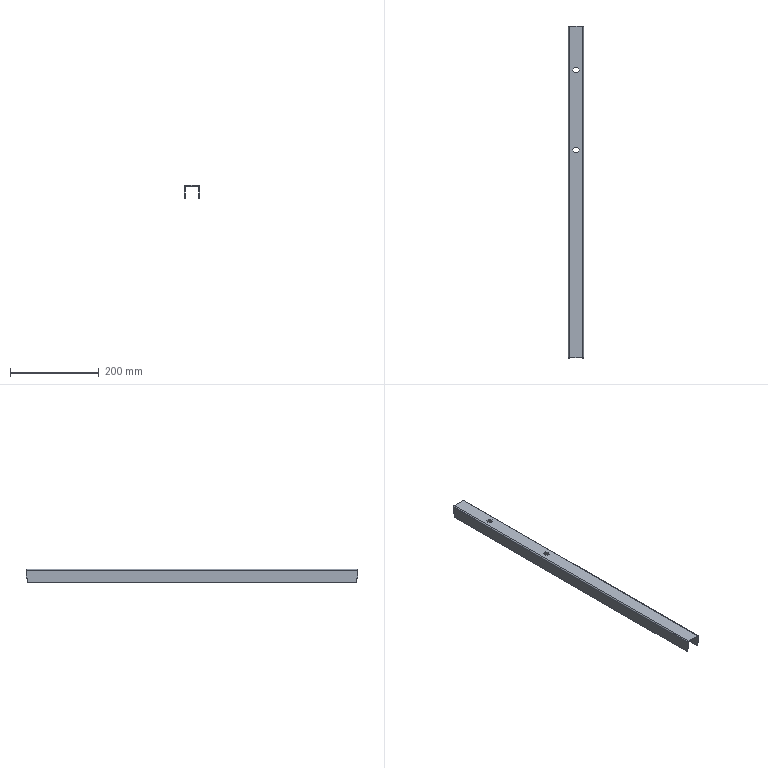Part | SolidWorks | features BaseBody 1 | 1 solid | 42 faces | box 34 x 750 x 29.5 mm | volume 130830 mm3 | plane 38 | cylinder 4 | commonest cylinder face diameters 1 x2 5 x2
STEP:
#1=CARTESIAN_POINT('',(-15.,372.,-29.5));
#2=VERTEX_POINT('',#1);
#3=CARTESIAN_POINT('',(-17.,372.,-29.5));
#4=VERTEX_POINT('',#3);
#5=CARTESIAN_POINT('',(17.,372.,-29.5));
#6=DIRECTION('',(-1.,0.,0.));
#7=VECTOR('',#6,1000.);
#8=LINE('',#5,#7);
#9=EDGE_CURVE('',#2,#4,#8,.T.);
#10=ORIENTED_EDGE('',*,*,#9,.T.);
#11=CARTESIAN_POINT('',(-17.,372.,-19.5));
#12=VERTEX_POINT('',#11);
#13=CARTESIAN_POINT('',(-17.,372.,-29.5));
#14=DIRECTION('',(0.,0.,1.));
#15=VECTOR('',#14,1000.);
#16=LINE('',#13,#15);
#17=EDGE_CURVE('',#4,#12,#16,.T.);
#18=ORIENTED_EDGE('',*,*,#17,.T.);
#19=CARTESIAN_POINT('',(-15.,372.,-19.5));
#20=VERTEX_POINT('',#19);
#21=CARTESIAN_POINT('',(17.,372.,-19.5));
#22=DIRECTION('',(-1.,0.,0.));
#23=VECTOR('',#22,1000.);
#24=LINE('',#21,#23);
#25=EDGE_CURVE('',#20,#12,#24,.T.);
#26=ORIENTED_EDGE('',*,*,#25,.F.);
#27=CARTESIAN_POINT('',(-15.,372.,0.));
#28=DIRECTION('',(0.,0.,1.));
#29=VECTOR('',#28,1000.);
#30=LINE('',#27,#29);
#31=EDGE_CURVE('',#2,#20,#30,.T.);
#32=ORIENTED_EDGE('',*,*,#31,.F.);
#33=EDGE_LOOP('',(#10,#18,#26,#32));
#34=FACE_OUTER_BOUND('',#33,.T.);
#35=CARTESIAN_POINT('',(17.,372.,-29.5));
#36=DIRECTION('',(0.,-1.,0.));
#37=DIRECTION('',(0.,0.,-1.));
#38=AXIS2_PLACEMENT_3D('',#35,#36,#37);
#39=PLANE('',#38);
#40=ADVANCED_FACE('',(#34),#39,.F.);
#41=ORIENTED_EDGE('',*,*,#25,.T.);
#42=CARTESIAN_POINT('',(-17.,375.,-19.5));
#43=VERTEX_POINT('',#42);
#44=CARTESIAN_POINT('',(-17.,375.,-19.5));
#45=DIRECTION('',(0.,1.,0.));
#46=VECTOR('',#45,1000.);
#47=LINE('',#44,#46);
#48=EDGE_CURVE('',#12,#43,#47,.T.);
#49=ORIENTED_EDGE('',*,*,#48,.T.);
#50=CARTESIAN_POINT('',(-15.,375.,-19.5));
#51=VERTEX_POINT('',#50);
#52=CARTESIAN_POINT('',(17.,375.,-19.5));
#53=DIRECTION('',(-1.,0.,0.));
#54=VECTOR('',#53,1000.);
#55=LINE('',#52,#54);
#56=EDGE_CURVE('',#51,#43,#55,.T.);
#57=ORIENTED_EDGE('',*,*,#56,.F.);
#58=CARTESIAN_POINT('',(-15.,0.,-19.5));
#59=DIRECTION('',(0.,1.,0.));
#60=VECTOR('',#59,1000.);
#61=LINE('',#58,#60);
#62=EDGE_CURVE('',#20,#51,#61,.T.);
#63=ORIENTED_EDGE('',*,*,#62,.F.);
#64=EDGE_LOOP('',(#41,#49,#57,#63));
#65=FACE_OUTER_BOUND('',#64,.T.);
#66=CARTESIAN_POINT('',(17.,375.,-19.5));
#67=DIRECTION('',(0.,0.,1.));
#68=DIRECTION('',(1.,0.,0.));
#69=AXIS2_PLACEMENT_3D('',#66,#67,#68);
#70=PLANE('',#69);
#71=ADVANCED_FACE('',(#65),#70,.F.);
#72=CARTESIAN_POINT('',(-15.,-372.,-19.5));
#73=VERTEX_POINT('',#72);
#74=CARTESIAN_POINT('',(-17.,-372.,-19.5));
#75=VERTEX_POINT('',#74);
#76=CARTESIAN_POINT('',(17.,-372.,-19.5));
#77=DIRECTION('',(-1.,0.,0.));
#78=VECTOR('',#77,1000.);
#79=LINE('',#76,#78);
#80=EDGE_CURVE('',#73,#75,#79,.T.);
#81=ORIENTED_EDGE('',*,*,#80,.T.);
#82=CARTESIAN_POINT('',(-17.,-372.,-29.5));
#83=VERTEX_POINT('',#82);
#84=CARTESIAN_POINT('',(-17.,-372.,-29.5));
#85=DIRECTION('',(0.,0.,-1.));
#86=VECTOR('',#85,1000.);
#87=LINE('',#84,#86);
#88=EDGE_CURVE('',#75,#83,#87,.T.);
#89=ORIENTED_EDGE('',*,*,#88,.T.);
#90=CARTESIAN_POINT('',(-15.,-372.,-29.5));
#91=VERTEX_POINT('',#90);
#92=CARTESIAN_POINT('',(17.,-372.,-29.5));
#93=DIRECTION('',(-1.,0.,0.));
#94=VECTOR('',#93,1000.);
#95=LINE('',#92,#94);
#96=EDGE_CURVE('',#91,#83,#95,.T.);
#97=ORIENTED_EDGE('',*,*,#96,.F.);
#98=CARTESIAN_POINT('',(-15.,-372.,0.));
#99=DIRECTION('',(0.,0.,-1.));
#100=VECTOR('',#99,1000.);
#101=LINE('',#98,#100);
#102=EDGE_CURVE('',#73,#91,#101,.T.);
#103=ORIENTED_EDGE('',*,*,#102,.F.);
#104=EDGE_LOOP('',(#81,#89,#97,#103));
#105=FACE_OUTER_BOUND('',#104,.T.);
#106=CARTESIAN_POINT('',(17.,-372.,-29.5));
#107=DIRECTION('',(0.,1.,0.));
#108=DIRECTION('',(1.,0.,0.));
#109=AXIS2_PLACEMENT_3D('',#106,#107,#108);
#110=PLANE('',#109);
#111=ADVANCED_FACE('',(#105),#110,.F.);
#112=CARTESIAN_POINT('',(-15.,-375.,-19.5));
#113=VERTEX_POINT('',#112);
#114=CARTESIAN_POINT('',(-17.,-375.,-19.5));
#115=VERTEX_POINT('',#114);
#116=CARTESIAN_POINT('',(17.,-375.,-19.5));
#117=DIRECTION('',(-1.,0.,0.));
#118=VECTOR('',#117,1000.);
#119=LINE('',#116,#118);
#120=EDGE_CURVE('',#113,#115,#119,.T.);
#121=ORIENTED_EDGE('',*,*,#120,.T.);
#122=CARTESIAN_POINT('',(-17.,-375.,-19.5));
#123=DIRECTION('',(0.,1.,0.));
#124=VECTOR('',#123,1000.);
#125=LINE('',#122,#124);
#126=EDGE_CURVE('',#115,#75,#125,.T.);
#127=ORIENTED_EDGE('',*,*,#126,.T.);
#128=ORIENTED_EDGE('',*,*,#80,.F.);
#129=CARTESIAN_POINT('',(-15.,0.,-19.5));
#130=DIRECTION('',(0.,1.,0.));
#131=VECTOR('',#130,1000.);
#132=LINE('',#129,#131);
#133=EDGE_CURVE('',#113,#73,#132,.T.);
#134=ORIENTED_EDGE('',*,*,#133,.F.);
#135=EDGE_LOOP('',(#121,#127,#128,#134));
#136=FACE_OUTER_BOUND('',#135,.T.);
#137=CARTESIAN_POINT('',(17.,-375.,-19.5));
#138=DIRECTION('',(0.,0.,1.));
#139=DIRECTION('',(1.,0.,0.));
#140=AXIS2_PLACEMENT_3D('',#137,#138,#139);
#141=PLANE('',#140);
#142=ADVANCED_FACE('',(#136),#141,.F.);
#143=CARTESIAN_POINT('',(15.,372.,-19.5));
#144=VERTEX_POINT('',#143);
#145=CARTESIAN_POINT('',(15.,375.,-19.5));
#146=VERTEX_POINT('',#145);
#147=CARTESIAN_POINT('',(15.,0.,-19.5));
#148=DIRECTION('',(0.,1.,0.));
#149=VECTOR('',#148,1000.);
#150=LINE('',#147,#149);
#151=EDGE_CURVE('',#144,#146,#150,.T.);
#152=ORIENTED_EDGE('',*,*,#151,.T.);
#153=CARTESIAN_POINT('',(17.,375.,-19.5));
#154=VERTEX_POINT('',#153);
#155=CARTESIAN_POINT('',(17.,375.,-19.5));
#156=DIRECTION('',(-1.,0.,0.));
#157=VECTOR('',#156,1000.);
#158=LINE('',#155,#157);
#159=EDGE_CURVE('',#154,#146,#158,.T.);
#160=ORIENTED_EDGE('',*,*,#159,.F.);
#161=CARTESIAN_POINT('',(17.,372.,-19.5));
#162=VERTEX_POINT('',#161);
#163=CARTESIAN_POINT('',(17.,375.,-19.5));
#164=DIRECTION('',(0.,1.,0.));
#165=VECTOR('',#164,1000.);
#166=LINE('',#163,#165);
#167=EDGE_CURVE('',#162,#154,#166,.T.);
#168=ORIENTED_EDGE('',*,*,#167,.F.);
#169=CARTESIAN_POINT('',(17.,372.,-19.5));
#170=DIRECTION('',(-1.,0.,0.));
#171=VECTOR('',#170,1000.);
#172=LINE('',#169,#171);
#173=EDGE_CURVE('',#162,#144,#172,.T.);
#174=ORIENTED_EDGE('',*,*,#173,.T.);
#175=EDGE_LOOP('',(#152,#160,#168,#174));
#176=FACE_OUTER_BOUND('',#175,.T.);
#177=CARTESIAN_POINT('',(17.,375.,-19.5));
#178=DIRECTION('',(0.,0.,1.));
#179=DIRECTION('',(1.,0.,0.));
#180=AXIS2_PLACEMENT_3D('',#177,#178,#179);
#181=PLANE('',#180);
#182=ADVANCED_FACE('',(#176),#181,.F.);
#183=CARTESIAN_POINT('',(15.,372.,-29.5));
#184=VERTEX_POINT('',#183);
#185=CARTESIAN_POINT('',(15.,372.,0.));
#186=DIRECTION('',(0.,0.,1.));
#187=VECTOR('',#186,1000.);
#188=LINE('',#185,#187);
#189=EDGE_CURVE('',#184,#144,#188,.T.);
#190=ORIENTED_EDGE('',*,*,#189,.T.);
#191=ORIENTED_EDGE('',*,*,#173,.F.);
#192=CARTESIAN_POINT('',(17.,372.,-29.5));
#193=VERTEX_POINT('',#192);
#194=CARTESIAN_POINT('',(17.,372.,-29.5));
#195=DIRECTION('',(0.,0.,1.));
#196=VECTOR('',#195,1000.);
#197=LINE('',#194,#196);
#198=EDGE_CURVE('',#193,#162,#197,.T.);
#199=ORIENTED_EDGE('',*,*,#198,.F.);
#200=CARTESIAN_POINT('',(17.,372.,-29.5));
#201=DIRECTION('',(-1.,0.,0.));
#202=VECTOR('',#201,1000.);
#203=LINE('',#200,#202);
#204=EDGE_CURVE('',#193,#184,#203,.T.);
#205=ORIENTED_EDGE('',*,*,#204,.T.);
#206=EDGE_LOOP('',(#190,#191,#199,#205));
#207=FACE_OUTER_BOUND('',#206,.T.);
#208=CARTESIAN_POINT('',(17.,372.,-29.5));
#209=DIRECTION('',(0.,-1.,0.));
#210=DIRECTION('',(0.,0.,-1.));
#211=AXIS2_PLACEMENT_3D('',#208,#209,#210);
#212=PLANE('',#211);
#213=ADVANCED_FACE('',(#207),#212,.F.);
#214=CARTESIAN_POINT('',(15.,-375.,-19.5));
#215=VERTEX_POINT('',#214);
#216=CARTESIAN_POINT('',(15.,-372.,-19.5));
#217=VERTEX_POINT('',#216);
#218=CARTESIAN_POINT('',(15.,0.,-19.5));
#219=DIRECTION('',(0.,1.,0.));
#220=VECTOR('',#219,1000.);
#221=LINE('',#218,#220);
#222=EDGE_CURVE('',#215,#217,#221,.T.);
#223=ORIENTED_EDGE('',*,*,#222,.T.);
#224=CARTESIAN_POINT('',(17.,-372.,-19.5));
#225=VERTEX_POINT('',#224);
#226=CARTESIAN_POINT('',(17.,-372.,-19.5));
#227=DIRECTION('',(-1.,0.,0.));
#228=VECTOR('',#227,1000.);
#229=LINE('',#226,#228);
#230=EDGE_CURVE('',#225,#217,#229,.T.);
#231=ORIENTED_EDGE('',*,*,#230,.F.);
#232=CARTESIAN_POINT('',(17.,-375.,-19.5));
#233=VERTEX_POINT('',#232);
#234=CARTESIAN_POINT('',(17.,-375.,-19.5));
#235=DIRECTION('',(0.,1.,0.));
#236=VECTOR('',#235,1000.);
#237=LINE('',#234,#236);
#238=EDGE_CURVE('',#233,#225,#237,.T.);
#239=ORIENTED_EDGE('',*,*,#238,.F.);
#240=CARTESIAN_POINT('',(17.,-375.,-19.5));
#241=DIRECTION('',(-1.,0.,0.));
#242=VECTOR('',#241,1000.);
#243=LINE('',#240,#242);
#244=EDGE_CURVE('',#233,#215,#243,.T.);
#245=ORIENTED_EDGE('',*,*,#244,.T.);
#246=EDGE_LOOP('',(#223,#231,#239,#245));
#247=FACE_OUTER_BOUND('',#246,.T.);
#248=CARTESIAN_POINT('',(17.,-375.,-19.5));
#249=DIRECTION('',(0.,0.,1.));
#250=DIRECTION('',(1.,0.,0.));
#251=AXIS2_PLACEMENT_3D('',#248,#249,#250);
#252=PLANE('',#251);
#253=ADVANCED_FACE('',(#247),#252,.F.);
#254=CARTESIAN_POINT('',(15.,-372.,-29.5));
#255=VERTEX_POINT('',#254);
#256=CARTESIAN_POINT('',(15.,-372.,0.));
#257=DIRECTION('',(0.,0.,-1.));
#258=VECTOR('',#257,1000.);
#259=LINE('',#256,#258);
#260=EDGE_CURVE('',#217,#255,#259,.T.);
#261=ORIENTED_EDGE('',*,*,#260,.T.);
#262=CARTESIAN_POINT('',(17.,-372.,-29.5));
#263=VERTEX_POINT('',#262);
#264=CARTESIAN_POINT('',(17.,-372.,-29.5));
#265=DIRECTION('',(-1.,0.,0.));
#266=VECTOR('',#265,1000.);
#267=LINE('',#264,#266);
#268=EDGE_CURVE('',#263,#255,#267,.T.);
#269=ORIENTED_EDGE('',*,*,#268,.F.);
#270=CARTESIAN_POINT('',(17.,-372.,-29.5));
#271=DIRECTION('',(0.,0.,-1.));
#272=VECTOR('',#271,1000.);
#273=LINE('',#270,#272);
#274=EDGE_CURVE('',#225,#263,#273,.T.);
#275=ORIENTED_EDGE('',*,*,#274,.F.);
#276=ORIENTED_EDGE('',*,*,#230,.T.);
#277=EDGE_LOOP('',(#261,#269,#275,#276));
#278=FACE_OUTER_BOUND('',#277,.T.);
#279=CARTESIAN_POINT('',(17.,-372.,-29.5));
#280=DIRECTION('',(0.,1.,0.));
#281=DIRECTION('',(1.,0.,0.));
#282=AXIS2_PLACEMENT_3D('',#279,#280,#281);
#283=PLANE('',#282);
#284=ADVANCED_FACE('',(#278),#283,.F.);
#285=CARTESIAN_POINT('',(6.928,275.,0.));
#286=VERTEX_POINT('',#285);
#287=CARTESIAN_POINT('',(3.464,281.,0.));
#288=VERTEX_POINT('',#287);
#289=CARTESIAN_POINT('',(6.928,275.,0.));
#290=DIRECTION('',(-0.5,0.866,0.));
#291=VECTOR('',#290,1000.);
#292=LINE('',#289,#291);
#293=EDGE_CURVE('',#286,#288,#292,.T.);
#294=ORIENTED_EDGE('',*,*,#293,.T.);
#295=CARTESIAN_POINT('',(3.464,281.,-2.));
#296=VERTEX_POINT('',#295);
#297=CARTESIAN_POINT('',(3.464,281.,-2.));
#298=DIRECTION('',(0.,0.,1.));
#299=VECTOR('',#298,1000.);
#300=LINE('',#297,#299);
#301=EDGE_CURVE('',#296,#288,#300,.T.);
#302=ORIENTED_EDGE('',*,*,#301,.F.);
#303=CARTESIAN_POINT('',(6.928,275.,-2.));
#304=VERTEX_POINT('',#303);
#305=CARTESIAN_POINT('',(6.928,275.,-2.));
#306=DIRECTION('',(-0.5,0.866,0.));
#307=VECTOR('',#306,1000.);
#308=LINE('',#305,#307);
#309=EDGE_CURVE('',#304,#296,#308,.T.);
#310=ORIENTED_EDGE('',*,*,#309,.F.);
#311=CARTESIAN_POINT('',(6.928,275.,-2.));
#312=DIRECTION('',(0.,0.,1.));
#313=VECTOR('',#312,1000.);
#314=LINE('',#311,#313);
#315=EDGE_CURVE('',#304,#286,#314,.T.);
#316=ORIENTED_EDGE('',*,*,#315,.T.);
#317=EDGE_LOOP('',(#294,#302,#310,#316));
#318=FACE_OUTER_BOUND('',#317,.T.);
#319=CARTESIAN_POINT('',(6.928,275.,-2.));
#320=DIRECTION('',(0.866,0.5,0.));
#321=DIRECTION('',(0.,0.,-1.));
#322=AXIS2_PLACEMENT_3D('',#319,#320,#321);
#323=PLANE('',#322);
#324=ADVANCED_FACE('',(#318),#323,.F.);
#325=CARTESIAN_POINT('',(-3.464,281.,0.));
#326=VERTEX_POINT('',#325);
#327=CARTESIAN_POINT('',(3.464,281.,0.));
#328=DIRECTION('',(-1.,0.,0.));
#329=VECTOR('',#328,1000.);
#330=LINE('',#327,#329);
#331=EDGE_CURVE('',#288,#326,#330,.T.);
#332=ORIENTED_EDGE('',*,*,#331,.T.);
#333=CARTESIAN_POINT('',(-3.464,281.,-2.));
#334=VERTEX_POINT('',#333);
#335=CARTESIAN_POINT('',(-3.464,281.,-2.));
#336=DIRECTION('',(0.,0.,1.));
#337=VECTOR('',#336,1000.);
#338=LINE('',#335,#337);
#339=EDGE_CURVE('',#334,#326,#338,.T.);
#340=ORIENTED_EDGE('',*,*,#339,.F.);
#341=CARTESIAN_POINT('',(3.464,281.,-2.));
#342=DIRECTION('',(-1.,0.,0.));
#343=VECTOR('',#342,1000.);
#344=LINE('',#341,#343);
#345=EDGE_CURVE('',#296,#334,#344,.T.);
#346=ORIENTED_EDGE('',*,*,#345,.F.);
#347=ORIENTED_EDGE('',*,*,#301,.T.);
#348=EDGE_LOOP('',(#332,#340,#346,#347));
#349=FACE_OUTER_BOUND('',#348,.T.);
#350=CARTESIAN_POINT('',(3.464,281.,-2.));
#351=DIRECTION('',(0.,1.,0.));
#352=DIRECTION('',(1.,0.,0.));
#353=AXIS2_PLACEMENT_3D('',#350,#351,#352);
#354=PLANE('',#353);
#355=ADVANCED_FACE('',(#349),#354,.F.);
#356=CARTESIAN_POINT('',(-6.928,275.,0.));
#357=VERTEX_POINT('',#356);
#358=CARTESIAN_POINT('',(-3.464,281.,0.));
#359=DIRECTION('',(-0.5,-0.866,0.));
#360=VECTOR('',#359,1000.);
#361=LINE('',#358,#360);
#362=EDGE_CURVE('',#326,#357,#361,.T.);
#363=ORIENTED_EDGE('',*,*,#362,.T.);
#364=CARTESIAN_POINT('',(-6.928,275.,-2.));
#365=VERTEX_POINT('',#364);
#366=CARTESIAN_POINT('',(-6.928,275.,-2.));
#367=DIRECTION('',(0.,0.,1.));
#368=VECTOR('',#367,1000.);
#369=LINE('',#366,#368);
#370=EDGE_CURVE('',#365,#357,#369,.T.);
#371=ORIENTED_EDGE('',*,*,#370,.F.);
#372=CARTESIAN_POINT('',(-3.464,281.,-2.));
#373=DIRECTION('',(-0.5,-0.866,0.));
#374=VECTOR('',#373,1000.);
#375=LINE('',#372,#374);
#376=EDGE_CURVE('',#334,#365,#375,.T.);
#377=ORIENTED_EDGE('',*,*,#376,.F.);
#378=ORIENTED_EDGE('',*,*,#339,.T.);
#379=EDGE_LOOP('',(#363,#371,#377,#378));
#380=FACE_OUTER_BOUND('',#379,.T.);
#381=CARTESIAN_POINT('',(-3.464,281.,-2.));
#382=DIRECTION('',(-0.866,0.5,0.));
#383=DIRECTION('',(0.,0.,1.));
#384=AXIS2_PLACEMENT_3D('',#381,#382,#383);
#385=PLANE('',#384);
#386=ADVANCED_FACE('',(#380),#385,.F.);
#387=CARTESIAN_POINT('',(-3.464,269.,0.));
#388=VERTEX_POINT('',#387);
#389=CARTESIAN_POINT('',(-6.928,275.,0.));
#390=DIRECTION('',(0.5,-0.866,0.));
#391=VECTOR('',#390,1000.);
#392=LINE('',#389,#391);
#393=EDGE_CURVE('',#357,#388,#392,.T.);
#394=ORIENTED_EDGE('',*,*,#393,.T.);
#395=CARTESIAN_POINT('',(-3.464,269.,-2.));
#396=VERTEX_POINT('',#395);
#397=CARTESIAN_POINT('',(-3.464,269.,-2.));
#398=DIRECTION('',(0.,0.,1.));
#399=VECTOR('',#398,1000.);
#400=LINE('',#397,#399);
#401=EDGE_CURVE('',#396,#388,#400,.T.);
#402=ORIENTED_EDGE('',*,*,#401,.F.);
#403=CARTESIAN_POINT('',(-6.928,275.,-2.));
#404=DIRECTION('',(0.5,-0.866,0.));
#405=VECTOR('',#404,1000.);
#406=LINE('',#403,#405);
#407=EDGE_CURVE('',#365,#396,#406,.T.);
#408=ORIENTED_EDGE('',*,*,#407,.F.);
#409=ORIENTED_EDGE('',*,*,#370,.T.);
#410=EDGE_LOOP('',(#394,#402,#408,#409));
#411=FACE_OUTER_BOUND('',#410,.T.);
#412=CARTESIAN_POINT('',(-6.928,275.,-2.));
#413=DIRECTION('',(-0.866,-0.5,0.));
#414=DIRECTION('',(-0.5,0.866,0.));
#415=AXIS2_PLACEMENT_3D('',#412,#413,#414);
#416=PLANE('',#415);
#417=ADVANCED_FACE('',(#411),#416,.F.);
#418=CARTESIAN_POINT('',(3.464,269.,0.));
#419=VERTEX_POINT('',#418);
#420=CARTESIAN_POINT('',(-3.464,269.,0.));
#421=DIRECTION('',(1.,0.,0.));
#422=VECTOR('',#421,1000.);
#423=LINE('',#420,#422);
#424=EDGE_CURVE('',#388,#419,#423,.T.);
#425=ORIENTED_EDGE('',*,*,#424,.T.);
#426=CARTESIAN_POINT('',(3.464,269.,-2.));
#427=VERTEX_POINT('',#426);
#428=CARTESIAN_POINT('',(3.464,269.,-2.));
#429=DIRECTION('',(0.,0.,1.));
#430=VECTOR('',#429,1000.);
#431=LINE('',#428,#430);
#432=EDGE_CURVE('',#427,#419,#431,.T.);
#433=ORIENTED_EDGE('',*,*,#432,.F.);
#434=CARTESIAN_POINT('',(-3.464,269.,-2.));
#435=DIRECTION('',(1.,0.,0.));
#436=VECTOR('',#435,1000.);
#437=LINE('',#434,#436);
#438=EDGE_CURVE('',#396,#427,#437,.T.);
#439=ORIENTED_EDGE('',*,*,#438,.F.);
#440=ORIENTED_EDGE('',*,*,#401,.T.);
#441=EDGE_LOOP('',(#425,#433,#439,#440));
#442=FACE_OUTER_BOUND('',#441,.T.);
#443=CARTESIAN_POINT('',(-3.464,269.,-2.));
#444=DIRECTION('',(0.,-1.,0.));
#445=DIRECTION('',(0.,0.,-1.));
#446=AXIS2_PLACEMENT_3D('',#443,#444,#445);
#447=PLANE('',#446);
#448=ADVANCED_FACE('',(#442),#447,.F.);
#449=CARTESIAN_POINT('',(3.464,269.,0.));
#450=DIRECTION('',(0.5,0.866,0.));
#451=VECTOR('',#450,1000.);
#452=LINE('',#449,#451);
#453=EDGE_CURVE('',#419,#286,#452,.T.);
#454=ORIENTED_EDGE('',*,*,#453,.T.);
#455=ORIENTED_EDGE('',*,*,#315,.F.);
#456=CARTESIAN_POINT('',(3.464,269.,-2.));
#457=DIRECTION('',(0.5,0.866,0.));
#458=VECTOR('',#457,1000.);
#459=LINE('',#456,#458);
#460=EDGE_CURVE('',#427,#304,#459,.T.);
#461=ORIENTED_EDGE('',*,*,#460,.F.);
#462=ORIENTED_EDGE('',*,*,#432,.T.);
#463=EDGE_LOOP('',(#454,#455,#461,#462));
#464=FACE_OUTER_BOUND('',#463,.T.);
#465=CARTESIAN_POINT('',(3.464,269.,-2.));
#466=DIRECTION('',(0.866,-0.5,0.));
#467=DIRECTION('',(0.,0.,-1.));
#468=AXIS2_PLACEMENT_3D('',#465,#466,#467);
#469=PLANE('',#468);
#470=ADVANCED_FACE('',(#464),#469,.F.);
#471=CARTESIAN_POINT('',(6.928,95.,0.));
#472=VERTEX_POINT('',#471);
#473=CARTESIAN_POINT('',(3.464,101.,0.));
#474=VERTEX_POINT('',#473);
#475=CARTESIAN_POINT('',(6.928,95.,0.));
#476=DIRECTION('',(-0.5,0.866,0.));
#477=VECTOR('',#476,1000.);
#478=LINE('',#475,#477);
#479=EDGE_CURVE('',#472,#474,#478,.T.);
#480=ORIENTED_EDGE('',*,*,#479,.T.);
#481=CARTESIAN_POINT('',(3.464,101.,-2.));
#482=VERTEX_POINT('',#481);
#483=CARTESIAN_POINT('',(3.464,101.,-2.));
#484=DIRECTION('',(0.,0.,1.));
#485=VECTOR('',#484,1000.);
#486=LINE('',#483,#485);
#487=EDGE_CURVE('',#482,#474,#486,.T.);
#488=ORIENTED_EDGE('',*,*,#487,.F.);
#489=CARTESIAN_POINT('',(6.928,95.,-2.));
#490=VERTEX_POINT('',#489);
#491=CARTESIAN_POINT('',(6.928,95.,-2.));
#492=DIRECTION('',(-0.5,0.866,0.));
#493=VECTOR('',#492,1000.);
#494=LINE('',#491,#493);
#495=EDGE_CURVE('',#490,#482,#494,.T.);
#496=ORIENTED_EDGE('',*,*,#495,.F.);
#497=CARTESIAN_POINT('',(6.928,95.,-2.));
#498=DIRECTION('',(0.,0.,1.));
#499=VECTOR('',#498,1000.);
#500=LINE('',#497,#499);
#501=EDGE_CURVE('',#490,#472,#500,.T.);
#502=ORIENTED_EDGE('',*,*,#501,.T.);
#503=EDGE_LOOP('',(#480,#488,#496,#502));
#504=FACE_OUTER_BOUND('',#503,.T.);
#505=CARTESIAN_POINT('',(6.928,95.,-2.));
#506=DIRECTION('',(0.866,0.5,0.));
#507=DIRECTION('',(0.,0.,-1.));
#508=AXIS2_PLACEMENT_3D('',#505,#506,#507);
#509=PLANE('',#508);
#510=ADVANCED_FACE('',(#504),#509,.F.);
#511=CARTESIAN_POINT('',(-3.464,101.,0.));
#512=VERTEX_POINT('',#511);
#513=CARTESIAN_POINT('',(3.464,101.,0.));
#514=DIRECTION('',(-1.,0.,0.));
#515=VECTOR('',#514,1000.);
#516=LINE('',#513,#515);
#517=EDGE_CURVE('',#474,#512,#516,.T.);
#518=ORIENTED_EDGE('',*,*,#517,.T.);
#519=CARTESIAN_POINT('',(-3.464,101.,-2.));
#520=VERTEX_POINT('',#519);
#521=CARTESIAN_POINT('',(-3.464,101.,-2.));
#522=DIRECTION('',(0.,0.,1.));
#523=VECTOR('',#522,1000.);
#524=LINE('',#521,#523);
#525=EDGE_CURVE('',#520,#512,#524,.T.);
#526=ORIENTED_EDGE('',*,*,#525,.F.);
#527=CARTESIAN_POINT('',(3.464,101.,-2.));
#528=DIRECTION('',(-1.,0.,0.));
#529=VECTOR('',#528,1000.);
#530=LINE('',#527,#529);
#531=EDGE_CURVE('',#482,#520,#530,.T.);
#532=ORIENTED_EDGE('',*,*,#531,.F.);
#533=ORIENTED_EDGE('',*,*,#487,.T.);
#534=EDGE_LOOP('',(#518,#526,#532,#533));
#535=FACE_OUTER_BOUND('',#534,.T.);
#536=CARTESIAN_POINT('',(3.464,101.,-2.));
#537=DIRECTION('',(0.,1.,0.));
#538=DIRECTION('',(1.,0.,0.));
#539=AXIS2_PLACEMENT_3D('',#536,#537,#538);
#540=PLANE('',#539);
#541=ADVANCED_FACE('',(#535),#540,.F.);
#542=CARTESIAN_POINT('',(-6.928,95.,0.));
#543=VERTEX_POINT('',#542);
#544=CARTESIAN_POINT('',(-3.464,101.,0.));
#545=DIRECTION('',(-0.5,-0.866,0.));
#546=VECTOR('',#545,1000.);
#547=LINE('',#544,#546);
#548=EDGE_CURVE('',#512,#543,#547,.T.);
#549=ORIENTED_EDGE('',*,*,#548,.T.);
#550=CARTESIAN_POINT('',(-6.928,95.,-2.));
#551=VERTEX_POINT('',#550);
#552=CARTESIAN_POINT('',(-6.928,95.,-2.));
#553=DIRECTION('',(0.,0.,1.));
#554=VECTOR('',#553,1000.);
#555=LINE('',#552,#554);
#556=EDGE_CURVE('',#551,#543,#555,.T.);
#557=ORIENTED_EDGE('',*,*,#556,.F.);
#558=CARTESIAN_POINT('',(-3.464,101.,-2.));
#559=DIRECTION('',(-0.5,-0.866,0.));
#560=VECTOR('',#559,1000.);
#561=LINE('',#558,#560);
#562=EDGE_CURVE('',#520,#551,#561,.T.);
#563=ORIENTED_EDGE('',*,*,#562,.F.);
#564=ORIENTED_EDGE('',*,*,#525,.T.);
#565=EDGE_LOOP('',(#549,#557,#563,#564));
#566=FACE_OUTER_BOUND('',#565,.T.);
#567=CARTESIAN_POINT('',(-3.464,101.,-2.));
#568=DIRECTION('',(-0.866,0.5,0.));
#569=DIRECTION('',(0.,0.,1.));
#570=AXIS2_PLACEMENT_3D('',#567,#568,#569);
#571=PLANE('',#570);
#572=ADVANCED_FACE('',(#566),#571,.F.);
#573=CARTESIAN_POINT('',(-3.464,89.,0.));
#574=VERTEX_POINT('',#573);
#575=CARTESIAN_POINT('',(-6.928,95.,0.));
#576=DIRECTION('',(0.5,-0.866,0.));
#577=VECTOR('',#576,1000.);
#578=LINE('',#575,#577);
#579=EDGE_CURVE('',#543,#574,#578,.T.);
#580=ORIENTED_EDGE('',*,*,#579,.T.);
#581=CARTESIAN_POINT('',(-3.464,89.,-2.));
#582=VERTEX_POINT('',#581);
#583=CARTESIAN_POINT('',(-3.464,89.,-2.));
#584=DIRECTION('',(0.,0.,1.));
#585=VECTOR('',#584,1000.);
#586=LINE('',#583,#585);
#587=EDGE_CURVE('',#582,#574,#586,.T.);
#588=ORIENTED_EDGE('',*,*,#587,.F.);
#589=CARTESIAN_POINT('',(-6.928,95.,-2.));
#590=DIRECTION('',(0.5,-0.866,0.));
#591=VECTOR('',#590,1000.);
#592=LINE('',#589,#591);
#593=EDGE_CURVE('',#551,#582,#592,.T.);
#594=ORIENTED_EDGE('',*,*,#593,.F.);
#595=ORIENTED_EDGE('',*,*,#556,.T.);
#596=EDGE_LOOP('',(#580,#588,#594,#595));
#597=FACE_OUTER_BOUND('',#596,.T.);
#598=CARTESIAN_POINT('',(-6.928,95.,-2.));
#599=DIRECTION('',(-0.866,-0.5,0.));
#600=DIRECTION('',(-0.5,0.866,0.));
#601=AXIS2_PLACEMENT_3D('',#598,#599,#600);
#602=PLANE('',#601);
#603=ADVANCED_FACE('',(#597),#602,.F.);
#604=CARTESIAN_POINT('',(3.464,89.,0.));
#605=VERTEX_POINT('',#604);
#606=CARTESIAN_POINT('',(-3.464,89.,0.));
#607=DIRECTION('',(1.,0.,0.));
#608=VECTOR('',#607,1000.);
#609=LINE('',#606,#608);
#610=EDGE_CURVE('',#574,#605,#609,.T.);
#611=ORIENTED_EDGE('',*,*,#610,.T.);
#612=CARTESIAN_POINT('',(3.464,89.,-2.));
#613=VERTEX_POINT('',#612);
#614=CARTESIAN_POINT('',(3.464,89.,-2.));
#615=DIRECTION('',(0.,0.,1.));
#616=VECTOR('',#615,1000.);
#617=LINE('',#614,#616);
#618=EDGE_CURVE('',#613,#605,#617,.T.);
#619=ORIENTED_EDGE('',*,*,#618,.F.);
#620=CARTESIAN_POINT('',(-3.464,89.,-2.));
#621=DIRECTION('',(1.,0.,0.));
#622=VECTOR('',#621,1000.);
#623=LINE('',#620,#622);
#624=EDGE_CURVE('',#582,#613,#623,.T.);
#625=ORIENTED_EDGE('',*,*,#624,.F.);
#626=ORIENTED_EDGE('',*,*,#587,.T.);
#627=EDGE_LOOP('',(#611,#619,#625,#626));
#628=FACE_OUTER_BOUND('',#627,.T.);
#629=CARTESIAN_POINT('',(-3.464,89.,-2.));
#630=DIRECTION('',(0.,-1.,0.));
#631=DIRECTION('',(0.,0.,-1.));
#632=AXIS2_PLACEMENT_3D('',#629,#630,#631);
#633=PLANE('',#632);
#634=ADVANCED_FACE('',(#628),#633,.F.);
#635=CARTESIAN_POINT('',(3.464,89.,0.));
#636=DIRECTION('',(0.5,0.866,0.));
#637=VECTOR('',#636,1000.);
#638=LINE('',#635,#637);
#639=EDGE_CURVE('',#605,#472,#638,.T.);
#640=ORIENTED_EDGE('',*,*,#639,.T.);
#641=ORIENTED_EDGE('',*,*,#501,.F.);
#642=CARTESIAN_POINT('',(3.464,89.,-2.));
#643=DIRECTION('',(0.5,0.866,0.));
#644=VECTOR('',#643,1000.);
#645=LINE('',#642,#644);
#646=EDGE_CURVE('',#613,#490,#645,.T.);
#647=ORIENTED_EDGE('',*,*,#646,.F.);
#648=ORIENTED_EDGE('',*,*,#618,.T.);
#649=EDGE_LOOP('',(#640,#641,#647,#648));
#650=FACE_OUTER_BOUND('',#649,.T.);
#651=CARTESIAN_POINT('',(3.464,89.,-2.));
#652=DIRECTION('',(0.866,-0.5,0.));
#653=DIRECTION('',(0.,0.,-1.));
#654=AXIS2_PLACEMENT_3D('',#651,#652,#653);
#655=PLANE('',#654);
#656=ADVANCED_FACE('',(#650),#655,.F.);
#657=ORIENTED_EDGE('',*,*,#204,.F.);
#658=CARTESIAN_POINT('',(17.,375.,-29.5));
#659=DIRECTION('',(0.,-1.,0.));
#660=VECTOR('',#659,1000.);
#661=LINE('',#658,#660);
#662=EDGE_CURVE('',#193,#263,#661,.T.);
#663=ORIENTED_EDGE('',*,*,#662,.T.);
#664=ORIENTED_EDGE('',*,*,#268,.T.);
#665=CARTESIAN_POINT('',(15.,375.,-29.5));
#666=DIRECTION('',(0.,-1.,0.));
#667=VECTOR('',#666,1000.);
#668=LINE('',#665,#667);
#669=EDGE_CURVE('',#184,#255,#668,.T.);
#670=ORIENTED_EDGE('',*,*,#669,.F.);
#671=EDGE_LOOP('',(#657,#663,#664,#670));
#672=FACE_OUTER_BOUND('',#671,.T.);
#673=CARTESIAN_POINT('',(17.,375.,-29.5));
#674=DIRECTION('',(0.,0.,-1.));
#675=DIRECTION('',(0.,-1.,0.));
#676=AXIS2_PLACEMENT_3D('',#673,#674,#675);
#677=PLANE('',#676);
#678=ADVANCED_FACE('',(#672),#677,.T.);
#679=ORIENTED_EDGE('',*,*,#151,.F.);
#680=ORIENTED_EDGE('',*,*,#189,.F.);
#681=ORIENTED_EDGE('',*,*,#669,.T.);
#682=ORIENTED_EDGE('',*,*,#260,.F.);
#683=ORIENTED_EDGE('',*,*,#222,.F.);
#684=CARTESIAN_POINT('',(15.,-375.,-2.5));
#685=VERTEX_POINT('',#684);
#686=CARTESIAN_POINT('',(15.,-375.,-29.5));
#687=DIRECTION('',(0.,0.,1.));
#688=VECTOR('',#687,1000.);
#689=LINE('',#686,#688);
#690=EDGE_CURVE('',#215,#685,#689,.T.);
#691=ORIENTED_EDGE('',*,*,#690,.T.);
#692=CARTESIAN_POINT('',(15.,375.,-2.5));
#693=VERTEX_POINT('',#692);
#694=CARTESIAN_POINT('',(15.,375.,-2.5));
#695=DIRECTION('',(0.,-1.,0.));
#696=VECTOR('',#695,1000.);
#697=LINE('',#694,#696);
#698=EDGE_CURVE('',#693,#685,#697,.T.);
#699=ORIENTED_EDGE('',*,*,#698,.F.);
#700=CARTESIAN_POINT('',(15.,375.,-2.));
#701=DIRECTION('',(0.,0.,-1.));
#702=VECTOR('',#701,1000.);
#703=LINE('',#700,#702);
#704=EDGE_CURVE('',#693,#146,#703,.T.);
#705=ORIENTED_EDGE('',*,*,#704,.T.);
#706=EDGE_LOOP('',(#679,#680,#681,#682,#683,#691,#699,#705));
#707=FACE_OUTER_BOUND('',#706,.T.);
#708=CARTESIAN_POINT('',(15.,0.,0.));
#709=DIRECTION('',(-1.,0.,0.));
#710=DIRECTION('',(0.,0.,1.));
#711=AXIS2_PLACEMENT_3D('',#708,#709,#710);
#712=PLANE('',#711);
#713=ADVANCED_FACE('',(#707),#712,.T.);
#714=ORIENTED_EDGE('',*,*,#198,.T.);
#715=ORIENTED_EDGE('',*,*,#167,.T.);
#716=CARTESIAN_POINT('',(17.,375.,-2.5));
#717=VERTEX_POINT('',#716);
#718=CARTESIAN_POINT('',(17.,375.,-2.));
#719=DIRECTION('',(0.,0.,-1.));
#720=VECTOR('',#719,1000.);
#721=LINE('',#718,#720);
#722=EDGE_CURVE('',#717,#154,#721,.T.);
#723=ORIENTED_EDGE('',*,*,#722,.F.);
#724=CARTESIAN_POINT('',(17.,-375.,-2.5));
#725=VERTEX_POINT('',#724);
#726=CARTESIAN_POINT('',(17.,0.,-2.5));
#727=DIRECTION('',(0.,1.,0.));
#728=VECTOR('',#727,1000.);
#729=LINE('',#726,#728);
#730=EDGE_CURVE('',#725,#717,#729,.T.);
#731=ORIENTED_EDGE('',*,*,#730,.F.);
#732=CARTESIAN_POINT('',(17.,-375.,-29.5));
#733=DIRECTION('',(0.,0.,1.));
#734=VECTOR('',#733,1000.);
#735=LINE('',#732,#734);
#736=EDGE_CURVE('',#233,#725,#735,.T.);
#737=ORIENTED_EDGE('',*,*,#736,.F.);
#738=ORIENTED_EDGE('',*,*,#238,.T.);
#739=ORIENTED_EDGE('',*,*,#274,.T.);
#740=ORIENTED_EDGE('',*,*,#662,.F.);
#741=EDGE_LOOP('',(#714,#715,#723,#731,#737,#738,#739,#740));
#742=FACE_OUTER_BOUND('',#741,.T.);
#743=CARTESIAN_POINT('',(17.,0.,0.));
#744=DIRECTION('',(-1.,0.,0.));
#745=DIRECTION('',(0.,0.,1.));
#746=AXIS2_PLACEMENT_3D('',#743,#744,#745);
#747=PLANE('',#746);
#748=ADVANCED_FACE('',(#742),#747,.F.);
#749=ORIENTED_EDGE('',*,*,#244,.F.);
#750=ORIENTED_EDGE('',*,*,#736,.T.);
#751=CARTESIAN_POINT('',(15.,-375.,-2.5));
#752=DIRECTION('',(1.,0.,0.));
#753=VECTOR('',#752,1000.);
#754=LINE('',#751,#753);
#755=EDGE_CURVE('',#685,#725,#754,.T.);
#756=ORIENTED_EDGE('',*,*,#755,.F.);
#757=ORIENTED_EDGE('',*,*,#690,.F.);
#758=EDGE_LOOP('',(#749,#750,#756,#757));
#759=FACE_OUTER_BOUND('',#758,.T.);
#760=CARTESIAN_POINT('',(17.,-375.,-29.5));
#761=DIRECTION('',(0.,-1.,0.));
#762=DIRECTION('',(0.,0.,-1.));
#763=AXIS2_PLACEMENT_3D('',#760,#761,#762);
#764=PLANE('',#763);
#765=ADVANCED_FACE('',(#759),#764,.T.);
#766=ORIENTED_EDGE('',*,*,#159,.T.);
#767=ORIENTED_EDGE('',*,*,#704,.F.);
#768=CARTESIAN_POINT('',(15.,375.,-2.5));
#769=DIRECTION('',(1.,0.,0.));
#770=VECTOR('',#769,1000.);
#771=LINE('',#768,#770);
#772=EDGE_CURVE('',#693,#717,#771,.T.);
#773=ORIENTED_EDGE('',*,*,#772,.T.);
#774=ORIENTED_EDGE('',*,*,#722,.T.);
#775=EDGE_LOOP('',(#766,#767,#773,#774));
#776=FACE_OUTER_BOUND('',#775,.T.);
#777=CARTESIAN_POINT('',(17.,375.,-2.));
#778=DIRECTION('',(0.,1.,0.));
#779=DIRECTION('',(1.,0.,0.));
#780=AXIS2_PLACEMENT_3D('',#777,#778,#779);
#781=PLANE('',#780);
#782=ADVANCED_FACE('',(#776),#781,.T.);
#783=CARTESIAN_POINT('',(14.5,-375.,-2.));
#784=VERTEX_POINT('',#783);
#785=CARTESIAN_POINT('',(14.5,375.,-2.));
#786=VERTEX_POINT('',#785);
#787=CARTESIAN_POINT('',(14.5,-375.,-2.));
#788=DIRECTION('',(0.,1.,0.));
#789=VECTOR('',#788,1000.);
#790=LINE('',#787,#789);
#791=EDGE_CURVE('',#784,#786,#790,.T.);
#792=ORIENTED_EDGE('',*,*,#791,.T.);
#793=CARTESIAN_POINT('',(14.5,375.,-2.5));
#794=DIRECTION('',(0.,1.,0.));
#795=DIRECTION('',(0.,0.,-1.));
#796=AXIS2_PLACEMENT_3D('',#793,#794,#795);
#797=CIRCLE('',#796,0.5);
#798=EDGE_CURVE('',#786,#693,#797,.T.);
#799=ORIENTED_EDGE('',*,*,#798,.T.);
#800=ORIENTED_EDGE('',*,*,#698,.T.);
#801=CARTESIAN_POINT('',(14.5,-375.,-2.5));
#802=DIRECTION('',(0.,-1.,0.));
#803=DIRECTION('',(0.,0.,-1.));
#804=AXIS2_PLACEMENT_3D('',#801,#802,#803);
#805=CIRCLE('',#804,0.5);
#806=EDGE_CURVE('',#685,#784,#805,.T.);
#807=ORIENTED_EDGE('',*,*,#806,.T.);
#808=EDGE_LOOP('',(#792,#799,#800,#807));
#809=FACE_OUTER_BOUND('',#808,.T.);
#810=CARTESIAN_POINT('',(14.5,-375.,-2.5));
#811=DIRECTION('',(0.,-1.,0.));
#812=DIRECTION('',(1.,0.,0.));
#813=AXIS2_PLACEMENT_3D('',#810,#811,#812);
#814=CYLINDRICAL_SURFACE('',#813,0.5);
#815=ADVANCED_FACE('',(#809),#814,.F.);
#816=CARTESIAN_POINT('',(14.5,-375.,0.));
#817=VERTEX_POINT('',#816);
#818=CARTESIAN_POINT('',(14.5,375.,0.));
#819=VERTEX_POINT('',#818);
#820=CARTESIAN_POINT('',(14.5,-375.,0.));
#821=DIRECTION('',(0.,1.,0.));
#822=VECTOR('',#821,1000.);
#823=LINE('',#820,#822);
#824=EDGE_CURVE('',#817,#819,#823,.T.);
#825=ORIENTED_EDGE('',*,*,#824,.F.);
#826=CARTESIAN_POINT('',(14.5,-375.,-2.5));
#827=DIRECTION('',(0.,-1.,0.));
#828=DIRECTION('',(0.,0.,-1.));
#829=AXIS2_PLACEMENT_3D('',#826,#827,#828);
#830=CIRCLE('',#829,2.5);
#831=EDGE_CURVE('',#725,#817,#830,.T.);
#832=ORIENTED_EDGE('',*,*,#831,.F.);
#833=ORIENTED_EDGE('',*,*,#730,.T.);
#834=CARTESIAN_POINT('',(14.5,375.,-2.5));
#835=DIRECTION('',(0.,1.,0.));
#836=DIRECTION('',(0.,0.,-1.));
#837=AXIS2_PLACEMENT_3D('',#834,#835,#836);
#838=CIRCLE('',#837,2.5);
#839=EDGE_CURVE('',#819,#717,#838,.T.);
#840=ORIENTED_EDGE('',*,*,#839,.F.);
#841=EDGE_LOOP('',(#825,#832,#833,#840));
#842=FACE_OUTER_BOUND('',#841,.T.);
#843=CARTESIAN_POINT('',(14.5,-375.,-2.5));
#844=DIRECTION('',(0.,-1.,0.));
#845=DIRECTION('',(1.,0.,0.));
#846=AXIS2_PLACEMENT_3D('',#843,#844,#845);
#847=CYLINDRICAL_SURFACE('',#846,2.5);
#848=ADVANCED_FACE('',(#842),#847,.T.);
#849=ORIENTED_EDGE('',*,*,#806,.F.);
#850=ORIENTED_EDGE('',*,*,#755,.T.);
#851=ORIENTED_EDGE('',*,*,#831,.T.);
#852=CARTESIAN_POINT('',(14.5,-375.,-2.));
#853=DIRECTION('',(0.,0.,1.));
#854=VECTOR('',#853,1000.);
#855=LINE('',#852,#854);
#856=EDGE_CURVE('',#784,#817,#855,.T.);
#857=ORIENTED_EDGE('',*,*,#856,.F.);
#858=EDGE_LOOP('',(#849,#850,#851,#857));
#859=FACE_OUTER_BOUND('',#858,.T.);
#860=CARTESIAN_POINT('',(14.5,-375.,-2.5));
#861=DIRECTION('',(0.,1.,0.));
#862=DIRECTION('',(1.,0.,0.));
#863=AXIS2_PLACEMENT_3D('',#860,#861,#862);
#864=PLANE('',#863);
#865=ADVANCED_FACE('',(#859),#864,.F.);
#866=ORIENTED_EDGE('',*,*,#772,.F.);
#867=ORIENTED_EDGE('',*,*,#798,.F.);
#868=CARTESIAN_POINT('',(14.5,375.,-2.));
#869=DIRECTION('',(0.,0.,1.));
#870=VECTOR('',#869,1000.);
#871=LINE('',#868,#870);
#872=EDGE_CURVE('',#786,#819,#871,.T.);
#873=ORIENTED_EDGE('',*,*,#872,.T.);
#874=ORIENTED_EDGE('',*,*,#839,.T.);
#875=EDGE_LOOP('',(#866,#867,#873,#874));
#876=FACE_OUTER_BOUND('',#875,.T.);
#877=CARTESIAN_POINT('',(14.5,375.,-2.5));
#878=DIRECTION('',(0.,1.,0.));
#879=DIRECTION('',(1.,0.,0.));
#880=AXIS2_PLACEMENT_3D('',#877,#878,#879);
#881=PLANE('',#880);
#882=ADVANCED_FACE('',(#876),#881,.T.);
#883=ORIENTED_EDGE('',*,*,#9,.F.);
#884=CARTESIAN_POINT('',(-15.,375.,-29.5));
#885=DIRECTION('',(0.,1.,0.));
#886=VECTOR('',#885,1000.);
#887=LINE('',#884,#886);
#888=EDGE_CURVE('',#91,#2,#887,.T.);
#889=ORIENTED_EDGE('',*,*,#888,.F.);
#890=ORIENTED_EDGE('',*,*,#96,.T.);
#891=CARTESIAN_POINT('',(-17.,375.,-29.5));
#892=DIRECTION('',(0.,1.,0.));
#893=VECTOR('',#892,1000.);
#894=LINE('',#891,#893);
#895=EDGE_CURVE('',#83,#4,#894,.T.);
#896=ORIENTED_EDGE('',*,*,#895,.T.);
#897=EDGE_LOOP('',(#883,#889,#890,#896));
#898=FACE_OUTER_BOUND('',#897,.T.);
#899=CARTESIAN_POINT('',(-17.,375.,-29.5));
#900=DIRECTION('',(0.,0.,-1.));
#901=DIRECTION('',(-1.,0.,0.));
#902=AXIS2_PLACEMENT_3D('',#899,#900,#901);
#903=PLANE('',#902);
#904=ADVANCED_FACE('',(#898),#903,.T.);
#905=ORIENTED_EDGE('',*,*,#31,.T.);
#906=ORIENTED_EDGE('',*,*,#62,.T.);
#907=CARTESIAN_POINT('',(-15.,375.,-2.5));
#908=VERTEX_POINT('',#907);
#909=CARTESIAN_POINT('',(-15.,375.,-2.));
#910=DIRECTION('',(0.,0.,1.));
#911=VECTOR('',#910,1000.);
#912=LINE('',#909,#911);
#913=EDGE_CURVE('',#51,#908,#912,.T.);
#914=ORIENTED_EDGE('',*,*,#913,.T.);
#915=CARTESIAN_POINT('',(-15.,-375.,-2.5));
#916=VERTEX_POINT('',#915);
#917=CARTESIAN_POINT('',(-15.,-375.,-2.5));
#918=DIRECTION('',(0.,1.,0.));
#919=VECTOR('',#918,1000.);
#920=LINE('',#917,#919);
#921=EDGE_CURVE('',#916,#908,#920,.T.);
#922=ORIENTED_EDGE('',*,*,#921,.F.);
#923=CARTESIAN_POINT('',(-15.,-375.,-29.5));
#924=DIRECTION('',(0.,0.,-1.));
#925=VECTOR('',#924,1000.);
#926=LINE('',#923,#925);
#927=EDGE_CURVE('',#916,#113,#926,.T.);
#928=ORIENTED_EDGE('',*,*,#927,.T.);
#929=ORIENTED_EDGE('',*,*,#133,.T.);
#930=ORIENTED_EDGE('',*,*,#102,.T.);
#931=ORIENTED_EDGE('',*,*,#888,.T.);
#932=EDGE_LOOP('',(#905,#906,#914,#922,#928,#929,#930,#931));
#933=FACE_OUTER_BOUND('',#932,.T.);
#934=CARTESIAN_POINT('',(-15.,0.,0.));
#935=DIRECTION('',(-1.,0.,0.));
#936=DIRECTION('',(0.,1.,0.));
#937=AXIS2_PLACEMENT_3D('',#934,#935,#936);
#938=PLANE('',#937);
#939=ADVANCED_FACE('',(#933),#938,.F.);
#940=ORIENTED_EDGE('',*,*,#48,.F.);
#941=ORIENTED_EDGE('',*,*,#17,.F.);
#942=ORIENTED_EDGE('',*,*,#895,.F.);
#943=ORIENTED_EDGE('',*,*,#88,.F.);
#944=ORIENTED_EDGE('',*,*,#126,.F.);
#945=CARTESIAN_POINT('',(-17.,-375.,-2.5));
#946=VERTEX_POINT('',#945);
#947=CARTESIAN_POINT('',(-17.,-375.,-29.5));
#948=DIRECTION('',(0.,0.,-1.));
#949=VECTOR('',#948,1000.);
#950=LINE('',#947,#949);
#951=EDGE_CURVE('',#946,#115,#950,.T.);
#952=ORIENTED_EDGE('',*,*,#951,.F.);
#953=CARTESIAN_POINT('',(-17.,375.,-2.5));
#954=VERTEX_POINT('',#953);
#955=CARTESIAN_POINT('',(-17.,0.,-2.5));
#956=DIRECTION('',(0.,1.,0.));
#957=VECTOR('',#956,1000.);
#958=LINE('',#955,#957);
#959=EDGE_CURVE('',#946,#954,#958,.T.);
#960=ORIENTED_EDGE('',*,*,#959,.T.);
#961=CARTESIAN_POINT('',(-17.,375.,-2.));
#962=DIRECTION('',(0.,0.,1.));
#963=VECTOR('',#962,1000.);
#964=LINE('',#961,#963);
#965=EDGE_CURVE('',#43,#954,#964,.T.);
#966=ORIENTED_EDGE('',*,*,#965,.F.);
#967=EDGE_LOOP('',(#940,#941,#942,#943,#944,#952,#960,#966));
#968=FACE_OUTER_BOUND('',#967,.T.);
#969=CARTESIAN_POINT('',(-17.,0.,0.));
#970=DIRECTION('',(-1.,0.,0.));
#971=DIRECTION('',(0.,1.,0.));
#972=AXIS2_PLACEMENT_3D('',#969,#970,#971);
#973=PLANE('',#972);
#974=ADVANCED_FACE('',(#968),#973,.T.);
#975=ORIENTED_EDGE('',*,*,#120,.F.);
#976=ORIENTED_EDGE('',*,*,#927,.F.);
#977=CARTESIAN_POINT('',(-15.,-375.,-2.5));
#978=DIRECTION('',(-1.,0.,0.));
#979=VECTOR('',#978,1000.);
#980=LINE('',#977,#979);
#981=EDGE_CURVE('',#916,#946,#980,.T.);
#982=ORIENTED_EDGE('',*,*,#981,.T.);
#983=ORIENTED_EDGE('',*,*,#951,.T.);
#984=EDGE_LOOP('',(#975,#976,#982,#983));
#985=FACE_OUTER_BOUND('',#984,.T.);
#986=CARTESIAN_POINT('',(-17.,-375.,-29.5));
#987=DIRECTION('',(0.,-1.,0.));
#988=DIRECTION('',(-1.,0.,0.));
#989=AXIS2_PLACEMENT_3D('',#986,#987,#988);
#990=PLANE('',#989);
#991=ADVANCED_FACE('',(#985),#990,.T.);
#992=ORIENTED_EDGE('',*,*,#56,.T.);
#993=ORIENTED_EDGE('',*,*,#965,.T.);
#994=CARTESIAN_POINT('',(-15.,375.,-2.5));
#995=DIRECTION('',(-1.,0.,0.));
#996=VECTOR('',#995,1000.);
#997=LINE('',#994,#996);
#998=EDGE_CURVE('',#908,#954,#997,.T.);
#999=ORIENTED_EDGE('',*,*,#998,.F.);
#1000=ORIENTED_EDGE('',*,*,#913,.F.);
#1001=EDGE_LOOP('',(#992,#993,#999,#1000));
#1002=FACE_OUTER_BOUND('',#1001,.T.);
#1003=CARTESIAN_POINT('',(-17.,375.,-2.));
#1004=DIRECTION('',(0.,1.,0.));
#1005=DIRECTION('',(0.,0.,-1.));
#1006=AXIS2_PLACEMENT_3D('',#1003,#1004,#1005);
#1007=PLANE('',#1006);
#1008=ADVANCED_FACE('',(#1002),#1007,.T.);
#1009=CARTESIAN_POINT('',(-14.5,375.,-2.));
#1010=VERTEX_POINT('',#1009);
#1011=CARTESIAN_POINT('',(-14.5,-375.,-2.));
#1012=VERTEX_POINT('',#1011);
#1013=CARTESIAN_POINT('',(-14.5,375.,-2.));
#1014=DIRECTION('',(0.,-1.,0.));
#1015=VECTOR('',#1014,1000.);
#1016=LINE('',#1013,#1015);
#1017=EDGE_CURVE('',#1010,#1012,#1016,.T.);
#1018=ORIENTED_EDGE('',*,*,#1017,.T.);
#1019=CARTESIAN_POINT('',(-14.5,-375.,-2.5));
#1020=DIRECTION('',(0.,-1.,0.));
#1021=DIRECTION('',(0.,0.,1.));
#1022=AXIS2_PLACEMENT_3D('',#1019,#1020,#1021);
#1023=CIRCLE('',#1022,0.5);
#1024=EDGE_CURVE('',#1012,#916,#1023,.T.);
#1025=ORIENTED_EDGE('',*,*,#1024,.T.);
#1026=ORIENTED_EDGE('',*,*,#921,.T.);
#1027=CARTESIAN_POINT('',(-14.5,375.,-2.5));
#1028=DIRECTION('',(0.,1.,0.));
#1029=DIRECTION('',(0.,0.,1.));
#1030=AXIS2_PLACEMENT_3D('',#1027,#1028,#1029);
#1031=CIRCLE('',#1030,0.5);
#1032=EDGE_CURVE('',#908,#1010,#1031,.T.);
#1033=ORIENTED_EDGE('',*,*,#1032,.T.);
#1034=EDGE_LOOP('',(#1018,#1025,#1026,#1033));
#1035=FACE_OUTER_BOUND('',#1034,.T.);
#1036=CARTESIAN_POINT('',(-14.5,375.,-2.5));
#1037=DIRECTION('',(0.,1.,0.));
#1038=DIRECTION('',(-1.,0.,0.));
#1039=AXIS2_PLACEMENT_3D('',#1036,#1037,#1038);
#1040=CYLINDRICAL_SURFACE('',#1039,0.5);
#1041=ADVANCED_FACE('',(#1035),#1040,.F.);
#1042=CARTESIAN_POINT('',(-14.5,375.,0.));
#1043=VERTEX_POINT('',#1042);
#1044=CARTESIAN_POINT('',(-14.5,-375.,0.));
#1045=VERTEX_POINT('',#1044);
#1046=CARTESIAN_POINT('',(-14.5,375.,0.));
#1047=DIRECTION('',(0.,-1.,0.));
#1048=VECTOR('',#1047,1000.);
#1049=LINE('',#1046,#1048);
#1050=EDGE_CURVE('',#1043,#1045,#1049,.T.);
#1051=ORIENTED_EDGE('',*,*,#1050,.F.);
#1052=CARTESIAN_POINT('',(-14.5,375.,-2.5));
#1053=DIRECTION('',(0.,1.,0.));
#1054=DIRECTION('',(0.,0.,1.));
#1055=AXIS2_PLACEMENT_3D('',#1052,#1053,#1054);
#1056=CIRCLE('',#1055,2.5);
#1057=EDGE_CURVE('',#954,#1043,#1056,.T.);
#1058=ORIENTED_EDGE('',*,*,#1057,.F.);
#1059=ORIENTED_EDGE('',*,*,#959,.F.);
#1060=CARTESIAN_POINT('',(-14.5,-375.,-2.5));
#1061=DIRECTION('',(0.,-1.,0.));
#1062=DIRECTION('',(0.,0.,1.));
#1063=AXIS2_PLACEMENT_3D('',#1060,#1061,#1062);
#1064=CIRCLE('',#1063,2.5);
#1065=EDGE_CURVE('',#1045,#946,#1064,.T.);
#1066=ORIENTED_EDGE('',*,*,#1065,.F.);
#1067=EDGE_LOOP('',(#1051,#1058,#1059,#1066));
#1068=FACE_OUTER_BOUND('',#1067,.T.);
#1069=CARTESIAN_POINT('',(-14.5,375.,-2.5));
#1070=DIRECTION('',(0.,1.,0.));
#1071=DIRECTION('',(-1.,0.,0.));
#1072=AXIS2_PLACEMENT_3D('',#1069,#1070,#1071);
#1073=CYLINDRICAL_SURFACE('',#1072,2.5);
#1074=ADVANCED_FACE('',(#1068),#1073,.T.);
#1075=ORIENTED_EDGE('',*,*,#1032,.F.);
#1076=ORIENTED_EDGE('',*,*,#998,.T.);
#1077=ORIENTED_EDGE('',*,*,#1057,.T.);
#1078=CARTESIAN_POINT('',(-14.5,375.,-2.));
#1079=DIRECTION('',(0.,0.,1.));
#1080=VECTOR('',#1079,1000.);
#1081=LINE('',#1078,#1080);
#1082=EDGE_CURVE('',#1010,#1043,#1081,.T.);
#1083=ORIENTED_EDGE('',*,*,#1082,.F.);
#1084=EDGE_LOOP('',(#1075,#1076,#1077,#1083));
#1085=FACE_OUTER_BOUND('',#1084,.T.);
#1086=CARTESIAN_POINT('',(-14.5,375.,-2.5));
#1087=DIRECTION('',(0.,-1.,0.));
#1088=DIRECTION('',(0.,0.,-1.));
#1089=AXIS2_PLACEMENT_3D('',#1086,#1087,#1088);
#1090=PLANE('',#1089);
#1091=ADVANCED_FACE('',(#1085),#1090,.F.);
#1092=ORIENTED_EDGE('',*,*,#981,.F.);
#1093=ORIENTED_EDGE('',*,*,#1024,.F.);
#1094=CARTESIAN_POINT('',(-14.5,-375.,-2.));
#1095=DIRECTION('',(0.,0.,1.));
#1096=VECTOR('',#1095,1000.);
#1097=LINE('',#1094,#1096);
#1098=EDGE_CURVE('',#1012,#1045,#1097,.T.);
#1099=ORIENTED_EDGE('',*,*,#1098,.T.);
#1100=ORIENTED_EDGE('',*,*,#1065,.T.);
#1101=EDGE_LOOP('',(#1092,#1093,#1099,#1100));
#1102=FACE_OUTER_BOUND('',#1101,.T.);
#1103=CARTESIAN_POINT('',(-14.5,-375.,-2.5));
#1104=DIRECTION('',(0.,-1.,0.));
#1105=DIRECTION('',(0.,0.,-1.));
#1106=AXIS2_PLACEMENT_3D('',#1103,#1104,#1105);
#1107=PLANE('',#1106);
#1108=ADVANCED_FACE('',(#1102),#1107,.T.);
#1109=ORIENTED_EDGE('',*,*,#872,.F.);
#1110=CARTESIAN_POINT('',(15.,375.,-2.));
#1111=DIRECTION('',(-1.,0.,0.));
#1112=VECTOR('',#1111,1000.);
#1113=LINE('',#1110,#1112);
#1114=EDGE_CURVE('',#786,#1010,#1113,.T.);
#1115=ORIENTED_EDGE('',*,*,#1114,.T.);
#1116=ORIENTED_EDGE('',*,*,#1082,.T.);
#1117=CARTESIAN_POINT('',(15.,375.,0.));
#1118=DIRECTION('',(-1.,0.,0.));
#1119=VECTOR('',#1118,1000.);
#1120=LINE('',#1117,#1119);
#1121=EDGE_CURVE('',#819,#1043,#1120,.T.);
#1122=ORIENTED_EDGE('',*,*,#1121,.F.);
#1123=EDGE_LOOP('',(#1109,#1115,#1116,#1122));
#1124=FACE_OUTER_BOUND('',#1123,.T.);
#1125=CARTESIAN_POINT('',(15.,375.,-2.));
#1126=DIRECTION('',(0.,1.,0.));
#1127=DIRECTION('',(1.,0.,0.));
#1128=AXIS2_PLACEMENT_3D('',#1125,#1126,#1127);
#1129=PLANE('',#1128);
#1130=ADVANCED_FACE('',(#1124),#1129,.T.);
#1131=CARTESIAN_POINT('',(15.,-375.,-2.));
#1132=DIRECTION('',(1.,0.,0.));
#1133=VECTOR('',#1132,1000.);
#1134=LINE('',#1131,#1133);
#1135=EDGE_CURVE('',#1012,#784,#1134,.T.);
#1136=ORIENTED_EDGE('',*,*,#1135,.T.);
#1137=ORIENTED_EDGE('',*,*,#856,.T.);
#1138=CARTESIAN_POINT('',(15.,-375.,0.));
#1139=DIRECTION('',(1.,0.,0.));
#1140=VECTOR('',#1139,1000.);
#1141=LINE('',#1138,#1140);
#1142=EDGE_CURVE('',#1045,#817,#1141,.T.);
#1143=ORIENTED_EDGE('',*,*,#1142,.F.);
#1144=ORIENTED_EDGE('',*,*,#1098,.F.);
#1145=EDGE_LOOP('',(#1136,#1137,#1143,#1144));
#1146=FACE_OUTER_BOUND('',#1145,.T.);
#1147=CARTESIAN_POINT('',(15.,-375.,-2.));
#1148=DIRECTION('',(0.,-1.,0.));
#1149=DIRECTION('',(0.,0.,-1.));
#1150=AXIS2_PLACEMENT_3D('',#1147,#1148,#1149);
#1151=PLANE('',#1150);
#1152=ADVANCED_FACE('',(#1146),#1151,.T.);
#1153=ORIENTED_EDGE('',*,*,#479,.F.);
#1154=ORIENTED_EDGE('',*,*,#639,.F.);
#1155=ORIENTED_EDGE('',*,*,#610,.F.);
#1156=ORIENTED_EDGE('',*,*,#579,.F.);
#1157=ORIENTED_EDGE('',*,*,#548,.F.);
#1158=ORIENTED_EDGE('',*,*,#517,.F.);
#1159=EDGE_LOOP('',(#1153,#1154,#1155,#1156,#1157,#1158));
#1160=FACE_BOUND('',#1159,.T.);
#1161=ORIENTED_EDGE('',*,*,#293,.F.);
#1162=ORIENTED_EDGE('',*,*,#453,.F.);
#1163=ORIENTED_EDGE('',*,*,#424,.F.);
#1164=ORIENTED_EDGE('',*,*,#393,.F.);
#1165=ORIENTED_EDGE('',*,*,#362,.F.);
#1166=ORIENTED_EDGE('',*,*,#331,.F.);
#1167=EDGE_LOOP('',(#1161,#1162,#1163,#1164,#1165,#1166));
#1168=FACE_BOUND('',#1167,.T.);
#1169=ORIENTED_EDGE('',*,*,#824,.T.);
#1170=ORIENTED_EDGE('',*,*,#1121,.T.);
#1171=ORIENTED_EDGE('',*,*,#1050,.T.);
#1172=ORIENTED_EDGE('',*,*,#1142,.T.);
#1173=EDGE_LOOP('',(#1169,#1170,#1171,#1172));
#1174=FACE_OUTER_BOUND('',#1173,.T.);
#1175=CARTESIAN_POINT('',(0.,0.,0.));
#1176=DIRECTION('',(0.,0.,-1.));
#1177=DIRECTION('',(0.,-1.,0.));
#1178=AXIS2_PLACEMENT_3D('',#1175,#1176,#1177);
#1179=PLANE('',#1178);
#1180=ADVANCED_FACE('',(#1160,#1168,#1174),#1179,.F.);
#1181=ORIENTED_EDGE('',*,*,#646,.T.);
#1182=ORIENTED_EDGE('',*,*,#495,.T.);
#1183=ORIENTED_EDGE('',*,*,#531,.T.);
#1184=ORIENTED_EDGE('',*,*,#562,.T.);
#1185=ORIENTED_EDGE('',*,*,#593,.T.);
#1186=ORIENTED_EDGE('',*,*,#624,.T.);
#1187=EDGE_LOOP('',(#1181,#1182,#1183,#1184,#1185,#1186));
#1188=FACE_BOUND('',#1187,.T.);
#1189=ORIENTED_EDGE('',*,*,#460,.T.);
#1190=ORIENTED_EDGE('',*,*,#309,.T.);
#1191=ORIENTED_EDGE('',*,*,#345,.T.);
#1192=ORIENTED_EDGE('',*,*,#376,.T.);
#1193=ORIENTED_EDGE('',*,*,#407,.T.);
#1194=ORIENTED_EDGE('',*,*,#438,.T.);
#1195=EDGE_LOOP('',(#1189,#1190,#1191,#1192,#1193,#1194));
#1196=FACE_BOUND('',#1195,.T.);
#1197=ORIENTED_EDGE('',*,*,#1114,.F.);
#1198=ORIENTED_EDGE('',*,*,#791,.F.);
#1199=ORIENTED_EDGE('',*,*,#1135,.F.);
#1200=ORIENTED_EDGE('',*,*,#1017,.F.);
#1201=EDGE_LOOP('',(#1197,#1198,#1199,#1200));
#1202=FACE_OUTER_BOUND('',#1201,.T.);
#1203=CARTESIAN_POINT('',(0.,0.,-2.));
#1204=DIRECTION('',(0.,0.,-1.));
#1205=DIRECTION('',(0.,-1.,0.));
#1206=AXIS2_PLACEMENT_3D('',#1203,#1204,#1205);
#1207=PLANE('',#1206);
#1208=ADVANCED_FACE('',(#1188,#1196,#1202),#1207,.T.);
#1209=CLOSED_SHELL('',(#40,#71,#111,#142,#182,#213,#253,#284,#324,#355,#386,#417,#448,#470,#510,#541,#572,#603,#634,#656,#678,#713,#748,#765,#782,#815,#848,#865,#882,#904,#939,#974,#991,#1008,#1041,#1074,#1091,#1108,#1130,#1152,#1180,#1208));
#1210=MANIFOLD_SOLID_BREP('',#1209);
#1211=CARTESIAN_POINT('',(0.,0.,0.));
#1212=DIRECTION('',(0.,0.,1.));
#1213=DIRECTION('',(1.,0.,0.));
#1214=AXIS2_PLACEMENT_3D('',#1211,#1212,#1213);
#1215=(LENGTH_UNIT()NAMED_UNIT(*)SI_UNIT(.MILLI.,.METRE.));
#1216=UNCERTAINTY_MEASURE_WITH_UNIT(LENGTH_MEASURE(0.00001),#1215,'','');
#1217=(NAMED_UNIT(*)PLANE_ANGLE_UNIT()SI_UNIT($,.RADIAN.));
#1218=(NAMED_UNIT(*)SI_UNIT($,.STERADIAN.)SOLID_ANGLE_UNIT());
#1219=(GEOMETRIC_REPRESENTATION_CONTEXT(3)GLOBAL_UNCERTAINTY_ASSIGNED_CONTEXT((#1216))GLOBAL_UNIT_ASSIGNED_CONTEXT((#1215,#1217,#1218))REPRESENTATION_CONTEXT('',''));
#1220=ADVANCED_BREP_SHAPE_REPRESENTATION('',(#1210,#1214),#1219);